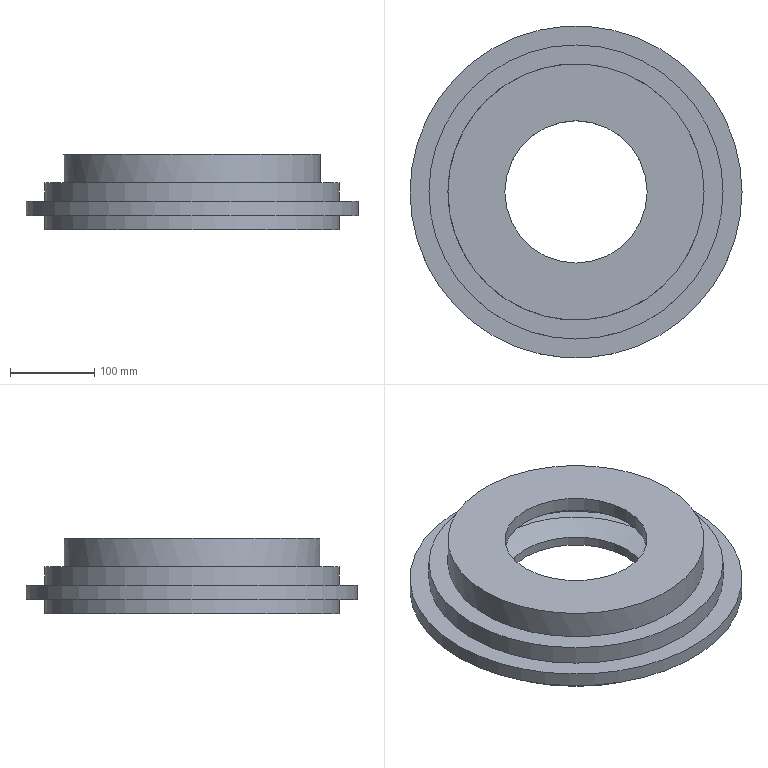Part | NX | features SIMPLE HOLE 4, CYLINDER 3, CHAMFER 2, DATUM_CSYS 1, Delete Body 1, LINKED_BODY 1, SCALE 1 | 1 solid | 18 faces | box 393.75 x 393.75 x 90 mm | volume 4276272 mm3 | cylinder 8 | plane 8 | cone 2 | commonest cylinder face diameters 168.75 x2 348.75 x2 258.75 x1 292.5 x1 303.75 x1 393.75 x1
STEP:
#1=CARTESIAN_POINT('',(-192.207,-1724.979,193.25));
#2=VERTEX_POINT('',#1);
#3=CARTESIAN_POINT('',(-366.582,-1724.979,193.25));
#4=DIRECTION('',(0.,0.,1.));
#5=DIRECTION('',(1.,0.,0.));
#6=AXIS2_PLACEMENT_3D('',#3,#4,#5);
#7=CIRCLE('',#6,174.375);
#8=EDGE_CURVE('',#2,#2,#7,.F.);
#9=ORIENTED_EDGE('',*,*,#8,.F.);
#10=EDGE_LOOP('',(#9));
#11=FACE_BOUND('',#10,.T.);
#12=CARTESIAN_POINT('',(-540.957,-1724.979,215.75));
#13=VERTEX_POINT('',#12);
#14=CARTESIAN_POINT('',(-366.582,-1724.979,215.75));
#15=DIRECTION('',(0.,0.,-1.));
#16=DIRECTION('',(-1.,0.,0.));
#17=AXIS2_PLACEMENT_3D('',#14,#15,#16);
#18=CIRCLE('',#17,174.375);
#19=EDGE_CURVE('',#13,#13,#18,.T.);
#20=ORIENTED_EDGE('',*,*,#19,.T.);
#21=EDGE_LOOP('',(#20));
#22=FACE_BOUND('',#21,.T.);
#23=CARTESIAN_POINT('',(-366.582,-1724.979,159.5));
#24=DIRECTION('',(0.,0.,1.));
#25=DIRECTION('',(1.,0.,0.));
#26=AXIS2_PLACEMENT_3D('',#23,#24,#25);
#27=CYLINDRICAL_SURFACE('',#26,174.375);
#28=ADVANCED_FACE('',(#11,#22),#27,.T.);
#29=CARTESIAN_POINT('',(-214.707,-1724.979,215.75));
#30=VERTEX_POINT('',#29);
#31=CARTESIAN_POINT('',(-366.582,-1724.979,215.75));
#32=DIRECTION('',(0.,0.,1.));
#33=DIRECTION('',(1.,0.,0.));
#34=AXIS2_PLACEMENT_3D('',#31,#32,#33);
#35=CIRCLE('',#34,151.875);
#36=EDGE_CURVE('',#30,#30,#35,.T.);
#37=ORIENTED_EDGE('',*,*,#36,.F.);
#38=EDGE_LOOP('',(#37));
#39=FACE_BOUND('',#38,.T.);
#40=ORIENTED_EDGE('',*,*,#19,.F.);
#41=EDGE_LOOP('',(#40));
#42=FACE_BOUND('',#41,.T.);
#43=CARTESIAN_POINT('',(-366.582,-1724.979,215.75));
#44=DIRECTION('',(0.,0.,1.));
#45=DIRECTION('',(1.,0.,0.));
#46=AXIS2_PLACEMENT_3D('',#43,#44,#45);
#47=PLANE('',#46);
#48=ADVANCED_FACE('',(#39,#42),#47,.T.);
#49=ORIENTED_EDGE('',*,*,#8,.T.);
#50=EDGE_LOOP('',(#49));
#51=FACE_BOUND('',#50,.T.);
#52=CARTESIAN_POINT('',(-563.457,-1724.979,193.25));
#53=VERTEX_POINT('',#52);
#54=CARTESIAN_POINT('',(-366.582,-1724.979,193.25));
#55=DIRECTION('',(0.,0.,-1.));
#56=DIRECTION('',(-1.,0.,0.));
#57=AXIS2_PLACEMENT_3D('',#54,#55,#56);
#58=CIRCLE('',#57,196.875);
#59=EDGE_CURVE('',#53,#53,#58,.T.);
#60=ORIENTED_EDGE('',*,*,#59,.F.);
#61=EDGE_LOOP('',(#60));
#62=FACE_BOUND('',#61,.T.);
#63=CARTESIAN_POINT('',(-366.582,-1724.979,193.25));
#64=DIRECTION('',(0.,0.,1.));
#65=DIRECTION('',(1.,0.,0.));
#66=AXIS2_PLACEMENT_3D('',#63,#64,#65);
#67=PLANE('',#66);
#68=ADVANCED_FACE('',(#51,#62),#67,.T.);
#69=CARTESIAN_POINT('',(-540.957,-1724.979,176.375));
#70=VERTEX_POINT('',#69);
#71=CARTESIAN_POINT('',(-366.582,-1724.979,176.375));
#72=DIRECTION('',(0.,0.,-1.));
#73=DIRECTION('',(-1.,0.,0.));
#74=AXIS2_PLACEMENT_3D('',#71,#72,#73);
#75=CIRCLE('',#74,174.375);
#76=EDGE_CURVE('',#70,#70,#75,.F.);
#77=ORIENTED_EDGE('',*,*,#76,.T.);
#78=EDGE_LOOP('',(#77));
#79=FACE_BOUND('',#78,.T.);
#80=CARTESIAN_POINT('',(-169.707,-1724.979,176.375));
#81=VERTEX_POINT('',#80);
#82=CARTESIAN_POINT('',(-366.582,-1724.979,176.375));
#83=DIRECTION('',(0.,0.,1.));
#84=DIRECTION('',(1.,0.,0.));
#85=AXIS2_PLACEMENT_3D('',#82,#83,#84);
#86=CIRCLE('',#85,196.875);
#87=EDGE_CURVE('',#81,#81,#86,.T.);
#88=ORIENTED_EDGE('',*,*,#87,.F.);
#89=EDGE_LOOP('',(#88));
#90=FACE_BOUND('',#89,.T.);
#91=CARTESIAN_POINT('',(-366.582,-1724.979,176.375));
#92=DIRECTION('',(0.,0.,-1.));
#93=DIRECTION('',(-1.,0.,0.));
#94=AXIS2_PLACEMENT_3D('',#91,#92,#93);
#95=PLANE('',#94);
#96=ADVANCED_FACE('',(#79,#90),#95,.T.);
#97=ORIENTED_EDGE('',*,*,#59,.T.);
#98=EDGE_LOOP('',(#97));
#99=FACE_BOUND('',#98,.T.);
#100=ORIENTED_EDGE('',*,*,#87,.T.);
#101=EDGE_LOOP('',(#100));
#102=FACE_BOUND('',#101,.T.);
#103=CARTESIAN_POINT('',(-366.582,-1724.979,176.375));
#104=DIRECTION('',(0.,0.,1.));
#105=DIRECTION('',(1.,0.,0.));
#106=AXIS2_PLACEMENT_3D('',#103,#104,#105);
#107=CYLINDRICAL_SURFACE('',#106,196.875);
#108=ADVANCED_FACE('',(#99,#102),#107,.T.);
#109=CARTESIAN_POINT('',(-220.332,-1724.979,159.5));
#110=VERTEX_POINT('',#109);
#111=CARTESIAN_POINT('',(-366.582,-1724.979,159.5));
#112=DIRECTION('',(0.,0.,1.));
#113=DIRECTION('',(1.,0.,0.));
#114=AXIS2_PLACEMENT_3D('',#111,#112,#113);
#115=CIRCLE('',#114,146.25);
#116=EDGE_CURVE('',#110,#110,#115,.T.);
#117=ORIENTED_EDGE('',*,*,#116,.T.);
#118=EDGE_LOOP('',(#117));
#119=FACE_BOUND('',#118,.T.);
#120=CARTESIAN_POINT('',(-192.207,-1724.979,159.5));
#121=VERTEX_POINT('',#120);
#122=CARTESIAN_POINT('',(-366.582,-1724.979,159.5));
#123=DIRECTION('',(0.,0.,1.));
#124=DIRECTION('',(1.,0.,0.));
#125=AXIS2_PLACEMENT_3D('',#122,#123,#124);
#126=CIRCLE('',#125,174.375);
#127=EDGE_CURVE('',#121,#121,#126,.T.);
#128=ORIENTED_EDGE('',*,*,#127,.F.);
#129=EDGE_LOOP('',(#128));
#130=FACE_BOUND('',#129,.T.);
#131=CARTESIAN_POINT('',(-366.582,-1724.979,159.5));
#132=DIRECTION('',(0.,0.,-1.));
#133=DIRECTION('',(-1.,0.,0.));
#134=AXIS2_PLACEMENT_3D('',#131,#132,#133);
#135=PLANE('',#134);
#136=ADVANCED_FACE('',(#119,#130),#135,.T.);
#137=ORIENTED_EDGE('',*,*,#76,.F.);
#138=EDGE_LOOP('',(#137));
#139=FACE_BOUND('',#138,.T.);
#140=ORIENTED_EDGE('',*,*,#127,.T.);
#141=EDGE_LOOP('',(#140));
#142=FACE_BOUND('',#141,.T.);
#143=CARTESIAN_POINT('',(-366.582,-1724.979,159.5));
#144=DIRECTION('',(0.,0.,1.));
#145=DIRECTION('',(1.,0.,0.));
#146=AXIS2_PLACEMENT_3D('',#143,#144,#145);
#147=CYLINDRICAL_SURFACE('',#146,174.375);
#148=ADVANCED_FACE('',(#139,#142),#147,.T.);
#149=CARTESIAN_POINT('',(-450.957,-1724.979,249.5));
#150=VERTEX_POINT('',#149);
#151=CARTESIAN_POINT('',(-366.582,-1724.979,249.5));
#152=DIRECTION('',(0.,0.,-1.));
#153=DIRECTION('',(-1.,0.,0.));
#154=AXIS2_PLACEMENT_3D('',#151,#152,#153);
#155=CIRCLE('',#154,84.375);
#156=EDGE_CURVE('',#150,#150,#155,.T.);
#157=ORIENTED_EDGE('',*,*,#156,.T.);
#158=EDGE_LOOP('',(#157));
#159=FACE_BOUND('',#158,.T.);
#160=CARTESIAN_POINT('',(-518.457,-1724.979,249.5));
#161=VERTEX_POINT('',#160);
#162=CARTESIAN_POINT('',(-366.582,-1724.979,249.5));
#163=DIRECTION('',(0.,0.,-1.));
#164=DIRECTION('',(-1.,0.,0.));
#165=AXIS2_PLACEMENT_3D('',#162,#163,#164);
#166=CIRCLE('',#165,151.875);
#167=EDGE_CURVE('',#161,#161,#166,.T.);
#168=ORIENTED_EDGE('',*,*,#167,.F.);
#169=EDGE_LOOP('',(#168));
#170=FACE_BOUND('',#169,.T.);
#171=CARTESIAN_POINT('',(-366.582,-1724.979,249.5));
#172=DIRECTION('',(0.,0.,1.));
#173=DIRECTION('',(1.,0.,0.));
#174=AXIS2_PLACEMENT_3D('',#171,#172,#173);
#175=PLANE('',#174);
#176=ADVANCED_FACE('',(#159,#170),#175,.T.);
#177=ORIENTED_EDGE('',*,*,#36,.T.);
#178=EDGE_LOOP('',(#177));
#179=FACE_BOUND('',#178,.T.);
#180=ORIENTED_EDGE('',*,*,#167,.T.);
#181=EDGE_LOOP('',(#180));
#182=FACE_BOUND('',#181,.T.);
#183=CARTESIAN_POINT('',(-366.582,-1724.979,159.5));
#184=DIRECTION('',(0.,0.,1.));
#185=DIRECTION('',(1.,0.,0.));
#186=AXIS2_PLACEMENT_3D('',#183,#184,#185);
#187=CYLINDRICAL_SURFACE('',#186,151.875);
#188=ADVANCED_FACE('',(#179,#182),#187,.T.);
#189=CARTESIAN_POINT('',(-282.207,-1724.979,232.625));
#190=VERTEX_POINT('',#189);
#191=CARTESIAN_POINT('',(-366.582,-1724.979,232.625));
#192=DIRECTION('',(0.,0.,1.));
#193=DIRECTION('',(1.,0.,0.));
#194=AXIS2_PLACEMENT_3D('',#191,#192,#193);
#195=CIRCLE('',#194,84.375);
#196=EDGE_CURVE('',#190,#190,#195,.F.);
#197=ORIENTED_EDGE('',*,*,#196,.T.);
#198=EDGE_LOOP('',(#197));
#199=FACE_BOUND('',#198,.T.);
#200=ORIENTED_EDGE('',*,*,#156,.F.);
#201=EDGE_LOOP('',(#200));
#202=FACE_BOUND('',#201,.T.);
#203=CARTESIAN_POINT('',(-366.582,-1724.979,249.5));
#204=DIRECTION('',(0.,0.,-1.));
#205=DIRECTION('',(-1.,0.,0.));
#206=AXIS2_PLACEMENT_3D('',#203,#204,#205);
#207=CYLINDRICAL_SURFACE('',#206,84.375);
#208=ADVANCED_FACE('',(#199,#202),#207,.F.);
#209=CARTESIAN_POINT('',(-282.207,-1724.979,182.));
#210=VERTEX_POINT('',#209);
#211=CARTESIAN_POINT('',(-366.582,-1724.979,182.));
#212=DIRECTION('',(0.,0.,1.));
#213=DIRECTION('',(1.,0.,0.));
#214=AXIS2_PLACEMENT_3D('',#211,#212,#213);
#215=CIRCLE('',#214,84.375);
#216=EDGE_CURVE('',#210,#210,#215,.T.);
#217=ORIENTED_EDGE('',*,*,#216,.T.);
#218=EDGE_LOOP('',(#217));
#219=FACE_BOUND('',#218,.T.);
#220=CARTESIAN_POINT('',(-220.332,-1724.979,182.));
#221=VERTEX_POINT('',#220);
#222=CARTESIAN_POINT('',(-366.582,-1724.979,182.));
#223=DIRECTION('',(0.,0.,1.));
#224=DIRECTION('',(1.,0.,0.));
#225=AXIS2_PLACEMENT_3D('',#222,#223,#224);
#226=CIRCLE('',#225,146.25);
#227=EDGE_CURVE('',#221,#221,#226,.F.);
#228=ORIENTED_EDGE('',*,*,#227,.T.);
#229=EDGE_LOOP('',(#228));
#230=FACE_BOUND('',#229,.T.);
#231=CARTESIAN_POINT('',(-366.582,-1724.979,182.));
#232=DIRECTION('',(0.,0.,1.));
#233=DIRECTION('',(1.,0.,0.));
#234=AXIS2_PLACEMENT_3D('',#231,#232,#233);
#235=PLANE('',#234);
#236=ADVANCED_FACE('',(#219,#230),#235,.F.);
#237=ORIENTED_EDGE('',*,*,#227,.F.);
#238=EDGE_LOOP('',(#237));
#239=FACE_BOUND('',#238,.T.);
#240=ORIENTED_EDGE('',*,*,#116,.F.);
#241=EDGE_LOOP('',(#240));
#242=FACE_BOUND('',#241,.T.);
#243=CARTESIAN_POINT('',(-366.582,-1724.979,159.5));
#244=DIRECTION('',(0.,0.,1.));
#245=DIRECTION('',(1.,0.,0.));
#246=AXIS2_PLACEMENT_3D('',#243,#244,#245);
#247=CYLINDRICAL_SURFACE('',#246,146.25);
#248=ADVANCED_FACE('',(#239,#242),#247,.F.);
#249=CARTESIAN_POINT('',(-450.957,-1724.979,193.25));
#250=VERTEX_POINT('',#249);
#251=CARTESIAN_POINT('',(-366.582,-1724.979,193.25));
#252=DIRECTION('',(0.,0.,-1.));
#253=DIRECTION('',(-1.,0.,0.));
#254=AXIS2_PLACEMENT_3D('',#251,#252,#253);
#255=CIRCLE('',#254,84.375);
#256=EDGE_CURVE('',#250,#250,#255,.F.);
#257=ORIENTED_EDGE('',*,*,#256,.T.);
#258=EDGE_LOOP('',(#257));
#259=FACE_BOUND('',#258,.T.);
#260=ORIENTED_EDGE('',*,*,#216,.F.);
#261=EDGE_LOOP('',(#260));
#262=FACE_BOUND('',#261,.T.);
#263=CARTESIAN_POINT('',(-366.582,-1724.979,182.));
#264=DIRECTION('',(0.,0.,1.));
#265=DIRECTION('',(1.,0.,0.));
#266=AXIS2_PLACEMENT_3D('',#263,#264,#265);
#267=CYLINDRICAL_SURFACE('',#266,84.375);
#268=ADVANCED_FACE('',(#259,#262),#267,.F.);
#269=CARTESIAN_POINT('',(-248.457,-1724.979,227.));
#270=VERTEX_POINT('',#269);
#271=CARTESIAN_POINT('',(-366.582,-1724.979,227.));
#272=DIRECTION('',(0.,0.,1.));
#273=DIRECTION('',(1.,0.,0.));
#274=AXIS2_PLACEMENT_3D('',#271,#272,#273);
#275=CIRCLE('',#274,118.125);
#276=EDGE_CURVE('',#270,#270,#275,.T.);
#277=ORIENTED_EDGE('',*,*,#276,.T.);
#278=EDGE_LOOP('',(#277));
#279=FACE_BOUND('',#278,.T.);
#280=CARTESIAN_POINT('',(-237.207,-1724.979,227.));
#281=VERTEX_POINT('',#280);
#282=CARTESIAN_POINT('',(-366.582,-1724.979,227.));
#283=DIRECTION('',(0.,0.,1.));
#284=DIRECTION('',(1.,0.,0.));
#285=AXIS2_PLACEMENT_3D('',#282,#283,#284);
#286=CIRCLE('',#285,129.375);
#287=EDGE_CURVE('',#281,#281,#286,.F.);
#288=ORIENTED_EDGE('',*,*,#287,.T.);
#289=EDGE_LOOP('',(#288));
#290=FACE_BOUND('',#289,.T.);
#291=CARTESIAN_POINT('',(-366.582,-1724.979,227.));
#292=DIRECTION('',(0.,0.,1.));
#293=DIRECTION('',(1.,0.,0.));
#294=AXIS2_PLACEMENT_3D('',#291,#292,#293);
#295=PLANE('',#294);
#296=ADVANCED_FACE('',(#279,#290),#295,.F.);
#297=CARTESIAN_POINT('',(-484.707,-1724.979,198.875));
#298=VERTEX_POINT('',#297);
#299=CARTESIAN_POINT('',(-366.582,-1724.979,198.875));
#300=DIRECTION('',(0.,0.,-1.));
#301=DIRECTION('',(-1.,0.,0.));
#302=AXIS2_PLACEMENT_3D('',#299,#300,#301);
#303=CIRCLE('',#302,118.125);
#304=EDGE_CURVE('',#298,#298,#303,.T.);
#305=ORIENTED_EDGE('',*,*,#304,.T.);
#306=EDGE_LOOP('',(#305));
#307=FACE_BOUND('',#306,.T.);
#308=CARTESIAN_POINT('',(-237.207,-1724.979,198.875));
#309=VERTEX_POINT('',#308);
#310=CARTESIAN_POINT('',(-366.582,-1724.979,198.875));
#311=DIRECTION('',(0.,0.,1.));
#312=DIRECTION('',(1.,0.,0.));
#313=AXIS2_PLACEMENT_3D('',#310,#311,#312);
#314=CIRCLE('',#313,129.375);
#315=EDGE_CURVE('',#309,#309,#314,.F.);
#316=ORIENTED_EDGE('',*,*,#315,.F.);
#317=EDGE_LOOP('',(#316));
#318=FACE_BOUND('',#317,.T.);
#319=CARTESIAN_POINT('',(-366.582,-1724.979,198.875));
#320=DIRECTION('',(0.,0.,-1.));
#321=DIRECTION('',(-1.,0.,0.));
#322=AXIS2_PLACEMENT_3D('',#319,#320,#321);
#323=PLANE('',#322);
#324=ADVANCED_FACE('',(#307,#318),#323,.F.);
#325=ORIENTED_EDGE('',*,*,#287,.F.);
#326=EDGE_LOOP('',(#325));
#327=FACE_BOUND('',#326,.T.);
#328=ORIENTED_EDGE('',*,*,#315,.T.);
#329=EDGE_LOOP('',(#328));
#330=FACE_BOUND('',#329,.T.);
#331=CARTESIAN_POINT('',(-366.582,-1724.979,198.875));
#332=DIRECTION('',(0.,0.,1.));
#333=DIRECTION('',(1.,0.,0.));
#334=AXIS2_PLACEMENT_3D('',#331,#332,#333);
#335=CYLINDRICAL_SURFACE('',#334,129.375);
#336=ADVANCED_FACE('',(#327,#330),#335,.F.);
#337=ORIENTED_EDGE('',*,*,#276,.F.);
#338=EDGE_LOOP('',(#337));
#339=FACE_BOUND('',#338,.T.);
#340=ORIENTED_EDGE('',*,*,#196,.F.);
#341=EDGE_LOOP('',(#340));
#342=FACE_BOUND('',#341,.T.);
#343=CARTESIAN_POINT('',(-366.582,-1724.979,232.625));
#344=DIRECTION('',(0.,0.,-1.));
#345=DIRECTION('',(-1.,0.,0.));
#346=AXIS2_PLACEMENT_3D('',#343,#344,#345);
#347=CONICAL_SURFACE('',#346,84.375,1.406);
#348=ADVANCED_FACE('',(#339,#342),#347,.F.);
#349=ORIENTED_EDGE('',*,*,#304,.F.);
#350=EDGE_LOOP('',(#349));
#351=FACE_BOUND('',#350,.T.);
#352=ORIENTED_EDGE('',*,*,#256,.F.);
#353=EDGE_LOOP('',(#352));
#354=FACE_BOUND('',#353,.T.);
#355=CARTESIAN_POINT('',(-366.582,-1724.979,193.25));
#356=DIRECTION('',(0.,0.,1.));
#357=DIRECTION('',(1.,0.,0.));
#358=AXIS2_PLACEMENT_3D('',#355,#356,#357);
#359=CONICAL_SURFACE('',#358,84.375,1.406);
#360=ADVANCED_FACE('',(#351,#354),#359,.F.);
#361=CLOSED_SHELL('',(#28,#48,#68,#96,#108,#136,#148,#176,#188,#208,#236,#248,#268,#296,#324,#336,#348,#360));
#362=MANIFOLD_SOLID_BREP('',#361);
#363=(LENGTH_UNIT()NAMED_UNIT(*)SI_UNIT(.MILLI.,.METRE.));
#364=UNCERTAINTY_MEASURE_WITH_UNIT(LENGTH_MEASURE(0.00001),#363,'','');
#365=(NAMED_UNIT(*)PLANE_ANGLE_UNIT()SI_UNIT($,.RADIAN.));
#366=(NAMED_UNIT(*)SI_UNIT($,.STERADIAN.)SOLID_ANGLE_UNIT());
#367=(GEOMETRIC_REPRESENTATION_CONTEXT(3)GLOBAL_UNCERTAINTY_ASSIGNED_CONTEXT((#364))GLOBAL_UNIT_ASSIGNED_CONTEXT((#363,#365,#366))REPRESENTATION_CONTEXT('',''));
#368=ADVANCED_BREP_SHAPE_REPRESENTATION('',(#362),#367);